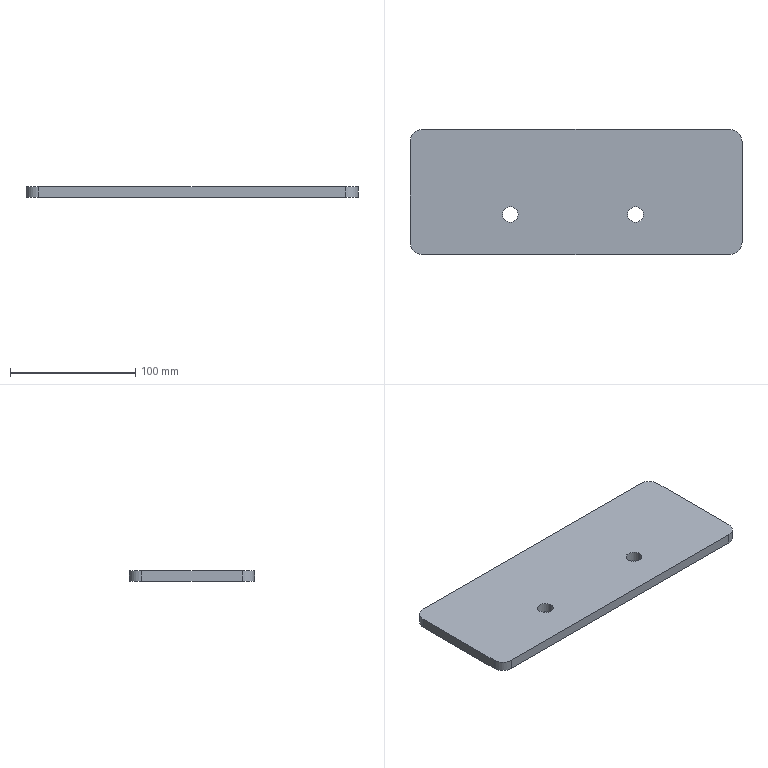Part | SolidWorks | features FlatPattern 1, ICE 1, SMBaseFlange 1, SheetMetal 1 | 1 solid | 103 faces | box 265 x 100 x 8 mm | volume 209194 mm3 | spline 76 | plane 19 | cylinder 8 | commonest cylinder face diameters 12.5 x4 20 x4